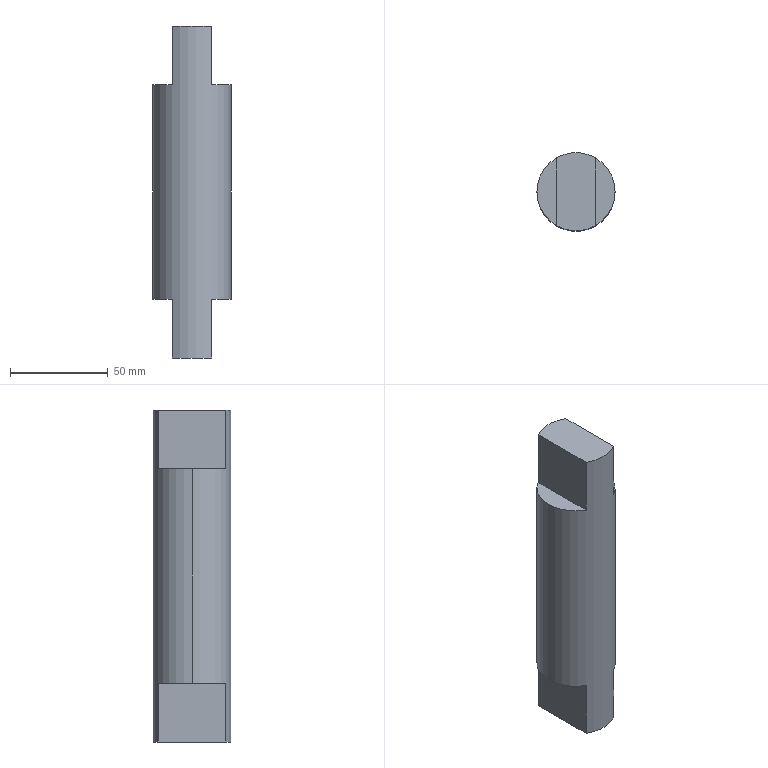Part | SolidWorks | 1 solid | 12 faces | box 40 x 40 x 170 mm | volume 184147 mm3 | plane 10 | cylinder 2 | commonest cylinder face diameters 40 x2
STEP:
#1=CARTESIAN_POINT('',(10.,17.321,0.));
#2=VERTEX_POINT('',#1);
#3=CARTESIAN_POINT('',(20.,0.,0.));
#4=VERTEX_POINT('',#3);
#5=CARTESIAN_POINT('',(0.,0.,0.));
#6=DIRECTION('',(0.,0.,-1.));
#7=DIRECTION('',(-1.,0.,0.));
#8=AXIS2_PLACEMENT_3D('',#5,#6,#7);
#9=CIRCLE('',#8,20.);
#10=EDGE_CURVE('',#2,#4,#9,.T.);
#11=ORIENTED_EDGE('',*,*,#10,.T.);
#12=CARTESIAN_POINT('',(20.,0.,-110.));
#13=VERTEX_POINT('',#12);
#14=CARTESIAN_POINT('',(20.,0.,30.));
#15=DIRECTION('',(0.,0.,-1.));
#16=VECTOR('',#15,1000.);
#17=LINE('',#14,#16);
#18=EDGE_CURVE('',#4,#13,#17,.T.);
#19=ORIENTED_EDGE('',*,*,#18,.T.);
#20=CARTESIAN_POINT('',(10.,17.321,-110.));
#21=VERTEX_POINT('',#20);
#22=CARTESIAN_POINT('',(0.,0.,-110.));
#23=DIRECTION('',(0.,0.,-1.));
#24=DIRECTION('',(-1.,0.,0.));
#25=AXIS2_PLACEMENT_3D('',#22,#23,#24);
#26=CIRCLE('',#25,20.);
#27=EDGE_CURVE('',#21,#13,#26,.T.);
#28=ORIENTED_EDGE('',*,*,#27,.F.);
#29=CARTESIAN_POINT('',(10.,17.321,-140.));
#30=VERTEX_POINT('',#29);
#31=CARTESIAN_POINT('',(10.,17.321,-140.));
#32=DIRECTION('',(0.,0.,1.));
#33=VECTOR('',#32,1000.);
#34=LINE('',#31,#33);
#35=EDGE_CURVE('',#30,#21,#34,.T.);
#36=ORIENTED_EDGE('',*,*,#35,.F.);
#37=CARTESIAN_POINT('',(-10.,17.321,-140.));
#38=VERTEX_POINT('',#37);
#39=CARTESIAN_POINT('',(0.,0.,-140.));
#40=DIRECTION('',(0.,0.,-1.));
#41=DIRECTION('',(-1.,0.,0.));
#42=AXIS2_PLACEMENT_3D('',#39,#40,#41);
#43=CIRCLE('',#42,20.);
#44=EDGE_CURVE('',#38,#30,#43,.T.);
#45=ORIENTED_EDGE('',*,*,#44,.F.);
#46=CARTESIAN_POINT('',(-10.,17.321,-110.));
#47=VERTEX_POINT('',#46);
#48=CARTESIAN_POINT('',(-10.,17.321,-140.));
#49=DIRECTION('',(0.,0.,1.));
#50=VECTOR('',#49,1000.);
#51=LINE('',#48,#50);
#52=EDGE_CURVE('',#38,#47,#51,.T.);
#53=ORIENTED_EDGE('',*,*,#52,.T.);
#54=CARTESIAN_POINT('',(-20.,0.,-110.));
#55=VERTEX_POINT('',#54);
#56=CARTESIAN_POINT('',(0.,0.,-110.));
#57=DIRECTION('',(0.,0.,-1.));
#58=DIRECTION('',(-1.,0.,0.));
#59=AXIS2_PLACEMENT_3D('',#56,#57,#58);
#60=CIRCLE('',#59,20.);
#61=EDGE_CURVE('',#55,#47,#60,.T.);
#62=ORIENTED_EDGE('',*,*,#61,.F.);
#63=CARTESIAN_POINT('',(-20.,0.,0.));
#64=VERTEX_POINT('',#63);
#65=CARTESIAN_POINT('',(-20.,0.,30.));
#66=DIRECTION('',(0.,0.,-1.));
#67=VECTOR('',#66,1000.);
#68=LINE('',#65,#67);
#69=EDGE_CURVE('',#64,#55,#68,.T.);
#70=ORIENTED_EDGE('',*,*,#69,.F.);
#71=CARTESIAN_POINT('',(-10.,17.321,0.));
#72=VERTEX_POINT('',#71);
#73=CARTESIAN_POINT('',(0.,0.,0.));
#74=DIRECTION('',(0.,0.,-1.));
#75=DIRECTION('',(-1.,0.,0.));
#76=AXIS2_PLACEMENT_3D('',#73,#74,#75);
#77=CIRCLE('',#76,20.);
#78=EDGE_CURVE('',#64,#72,#77,.T.);
#79=ORIENTED_EDGE('',*,*,#78,.T.);
#80=CARTESIAN_POINT('',(-10.,17.321,30.));
#81=VERTEX_POINT('',#80);
#82=CARTESIAN_POINT('',(-10.,17.321,30.));
#83=DIRECTION('',(0.,0.,-1.));
#84=VECTOR('',#83,1000.);
#85=LINE('',#82,#84);
#86=EDGE_CURVE('',#81,#72,#85,.T.);
#87=ORIENTED_EDGE('',*,*,#86,.F.);
#88=CARTESIAN_POINT('',(10.,17.321,30.));
#89=VERTEX_POINT('',#88);
#90=CARTESIAN_POINT('',(0.,0.,30.));
#91=DIRECTION('',(0.,0.,1.));
#92=DIRECTION('',(1.,0.,0.));
#93=AXIS2_PLACEMENT_3D('',#90,#91,#92);
#94=CIRCLE('',#93,20.);
#95=EDGE_CURVE('',#89,#81,#94,.T.);
#96=ORIENTED_EDGE('',*,*,#95,.F.);
#97=CARTESIAN_POINT('',(10.,17.321,30.));
#98=DIRECTION('',(0.,0.,-1.));
#99=VECTOR('',#98,1000.);
#100=LINE('',#97,#99);
#101=EDGE_CURVE('',#89,#2,#100,.T.);
#102=ORIENTED_EDGE('',*,*,#101,.T.);
#103=EDGE_LOOP('',(#11,#19,#28,#36,#45,#53,#62,#70,#79,#87,#96,#102));
#104=FACE_OUTER_BOUND('',#103,.T.);
#105=CARTESIAN_POINT('',(0.,0.,30.));
#106=DIRECTION('',(0.,0.,-1.));
#107=DIRECTION('',(-1.,0.,0.));
#108=AXIS2_PLACEMENT_3D('',#105,#106,#107);
#109=CYLINDRICAL_SURFACE('',#108,20.);
#110=ADVANCED_FACE('',(#104),#109,.T.);
#111=CARTESIAN_POINT('',(-10.,-17.321,-110.));
#112=VERTEX_POINT('',#111);
#113=CARTESIAN_POINT('',(0.,0.,-110.));
#114=DIRECTION('',(0.,0.,-1.));
#115=DIRECTION('',(-1.,0.,0.));
#116=AXIS2_PLACEMENT_3D('',#113,#114,#115);
#117=CIRCLE('',#116,20.);
#118=EDGE_CURVE('',#112,#55,#117,.T.);
#119=ORIENTED_EDGE('',*,*,#118,.T.);
#120=ORIENTED_EDGE('',*,*,#61,.T.);
#121=CARTESIAN_POINT('',(-10.,0.,-110.));
#122=DIRECTION('',(0.,-1.,0.));
#123=VECTOR('',#122,1000.);
#124=LINE('',#121,#123);
#125=EDGE_CURVE('',#47,#112,#124,.T.);
#126=ORIENTED_EDGE('',*,*,#125,.T.);
#127=EDGE_LOOP('',(#119,#120,#126));
#128=FACE_OUTER_BOUND('',#127,.T.);
#129=CARTESIAN_POINT('',(0.,0.,-110.));
#130=DIRECTION('',(0.,0.,-1.));
#131=DIRECTION('',(-1.,0.,0.));
#132=AXIS2_PLACEMENT_3D('',#129,#130,#131);
#133=PLANE('',#132);
#134=ADVANCED_FACE('',(#128),#133,.T.);
#135=CARTESIAN_POINT('',(-10.,-17.321,0.));
#136=VERTEX_POINT('',#135);
#137=CARTESIAN_POINT('',(-10.,0.,0.));
#138=DIRECTION('',(0.,-1.,0.));
#139=VECTOR('',#138,1000.);
#140=LINE('',#137,#139);
#141=EDGE_CURVE('',#72,#136,#140,.T.);
#142=ORIENTED_EDGE('',*,*,#141,.T.);
#143=CARTESIAN_POINT('',(-10.,-17.321,30.));
#144=VERTEX_POINT('',#143);
#145=CARTESIAN_POINT('',(-10.,-17.321,30.));
#146=DIRECTION('',(0.,0.,-1.));
#147=VECTOR('',#146,1000.);
#148=LINE('',#145,#147);
#149=EDGE_CURVE('',#144,#136,#148,.T.);
#150=ORIENTED_EDGE('',*,*,#149,.F.);
#151=CARTESIAN_POINT('',(-10.,0.,30.));
#152=DIRECTION('',(0.,-1.,0.));
#153=VECTOR('',#152,1000.);
#154=LINE('',#151,#153);
#155=EDGE_CURVE('',#81,#144,#154,.T.);
#156=ORIENTED_EDGE('',*,*,#155,.F.);
#157=ORIENTED_EDGE('',*,*,#86,.T.);
#158=EDGE_LOOP('',(#142,#150,#156,#157));
#159=FACE_OUTER_BOUND('',#158,.T.);
#160=CARTESIAN_POINT('',(-10.,0.,30.));
#161=DIRECTION('',(1.,0.,0.));
#162=DIRECTION('',(0.,0.,-1.));
#163=AXIS2_PLACEMENT_3D('',#160,#161,#162);
#164=PLANE('',#163);
#165=ADVANCED_FACE('',(#159),#164,.F.);
#166=ORIENTED_EDGE('',*,*,#18,.F.);
#167=CARTESIAN_POINT('',(10.,-17.321,0.));
#168=VERTEX_POINT('',#167);
#169=CARTESIAN_POINT('',(0.,0.,0.));
#170=DIRECTION('',(0.,0.,-1.));
#171=DIRECTION('',(-1.,0.,0.));
#172=AXIS2_PLACEMENT_3D('',#169,#170,#171);
#173=CIRCLE('',#172,20.);
#174=EDGE_CURVE('',#4,#168,#173,.T.);
#175=ORIENTED_EDGE('',*,*,#174,.T.);
#176=CARTESIAN_POINT('',(10.,-17.321,30.));
#177=VERTEX_POINT('',#176);
#178=CARTESIAN_POINT('',(10.,-17.321,30.));
#179=DIRECTION('',(0.,0.,-1.));
#180=VECTOR('',#179,1000.);
#181=LINE('',#178,#180);
#182=EDGE_CURVE('',#177,#168,#181,.T.);
#183=ORIENTED_EDGE('',*,*,#182,.F.);
#184=CARTESIAN_POINT('',(0.,0.,30.));
#185=DIRECTION('',(0.,0.,1.));
#186=DIRECTION('',(1.,0.,0.));
#187=AXIS2_PLACEMENT_3D('',#184,#185,#186);
#188=CIRCLE('',#187,20.);
#189=EDGE_CURVE('',#144,#177,#188,.T.);
#190=ORIENTED_EDGE('',*,*,#189,.F.);
#191=ORIENTED_EDGE('',*,*,#149,.T.);
#192=CARTESIAN_POINT('',(0.,0.,0.));
#193=DIRECTION('',(0.,0.,-1.));
#194=DIRECTION('',(-1.,0.,0.));
#195=AXIS2_PLACEMENT_3D('',#192,#193,#194);
#196=CIRCLE('',#195,20.);
#197=EDGE_CURVE('',#136,#64,#196,.T.);
#198=ORIENTED_EDGE('',*,*,#197,.T.);
#199=ORIENTED_EDGE('',*,*,#69,.T.);
#200=ORIENTED_EDGE('',*,*,#118,.F.);
#201=CARTESIAN_POINT('',(-10.,-17.321,-140.));
#202=VERTEX_POINT('',#201);
#203=CARTESIAN_POINT('',(-10.,-17.321,-140.));
#204=DIRECTION('',(0.,0.,1.));
#205=VECTOR('',#204,1000.);
#206=LINE('',#203,#205);
#207=EDGE_CURVE('',#202,#112,#206,.T.);
#208=ORIENTED_EDGE('',*,*,#207,.F.);
#209=CARTESIAN_POINT('',(10.,-17.321,-140.));
#210=VERTEX_POINT('',#209);
#211=CARTESIAN_POINT('',(0.,0.,-140.));
#212=DIRECTION('',(0.,0.,-1.));
#213=DIRECTION('',(-1.,0.,0.));
#214=AXIS2_PLACEMENT_3D('',#211,#212,#213);
#215=CIRCLE('',#214,20.);
#216=EDGE_CURVE('',#210,#202,#215,.T.);
#217=ORIENTED_EDGE('',*,*,#216,.F.);
#218=CARTESIAN_POINT('',(10.,-17.321,-110.));
#219=VERTEX_POINT('',#218);
#220=CARTESIAN_POINT('',(10.,-17.321,-140.));
#221=DIRECTION('',(0.,0.,1.));
#222=VECTOR('',#221,1000.);
#223=LINE('',#220,#222);
#224=EDGE_CURVE('',#210,#219,#223,.T.);
#225=ORIENTED_EDGE('',*,*,#224,.T.);
#226=CARTESIAN_POINT('',(0.,0.,-110.));
#227=DIRECTION('',(0.,0.,-1.));
#228=DIRECTION('',(-1.,0.,0.));
#229=AXIS2_PLACEMENT_3D('',#226,#227,#228);
#230=CIRCLE('',#229,20.);
#231=EDGE_CURVE('',#13,#219,#230,.T.);
#232=ORIENTED_EDGE('',*,*,#231,.F.);
#233=EDGE_LOOP('',(#166,#175,#183,#190,#191,#198,#199,#200,#208,#217,#225,#232));
#234=FACE_OUTER_BOUND('',#233,.T.);
#235=CARTESIAN_POINT('',(0.,0.,30.));
#236=DIRECTION('',(0.,0.,-1.));
#237=DIRECTION('',(-1.,0.,0.));
#238=AXIS2_PLACEMENT_3D('',#235,#236,#237);
#239=CYLINDRICAL_SURFACE('',#238,20.);
#240=ADVANCED_FACE('',(#234),#239,.T.);
#241=CARTESIAN_POINT('',(10.,0.,0.));
#242=DIRECTION('',(0.,-1.,0.));
#243=VECTOR('',#242,1000.);
#244=LINE('',#241,#243);
#245=EDGE_CURVE('',#2,#168,#244,.T.);
#246=ORIENTED_EDGE('',*,*,#245,.F.);
#247=ORIENTED_EDGE('',*,*,#101,.F.);
#248=CARTESIAN_POINT('',(10.,0.,30.));
#249=DIRECTION('',(0.,-1.,0.));
#250=VECTOR('',#249,1000.);
#251=LINE('',#248,#250);
#252=EDGE_CURVE('',#89,#177,#251,.T.);
#253=ORIENTED_EDGE('',*,*,#252,.T.);
#254=ORIENTED_EDGE('',*,*,#182,.T.);
#255=EDGE_LOOP('',(#246,#247,#253,#254));
#256=FACE_OUTER_BOUND('',#255,.T.);
#257=CARTESIAN_POINT('',(10.,0.,30.));
#258=DIRECTION('',(1.,0.,0.));
#259=DIRECTION('',(0.,0.,-1.));
#260=AXIS2_PLACEMENT_3D('',#257,#258,#259);
#261=PLANE('',#260);
#262=ADVANCED_FACE('',(#256),#261,.T.);
#263=ORIENTED_EDGE('',*,*,#95,.T.);
#264=ORIENTED_EDGE('',*,*,#155,.T.);
#265=ORIENTED_EDGE('',*,*,#189,.T.);
#266=ORIENTED_EDGE('',*,*,#252,.F.);
#267=EDGE_LOOP('',(#263,#264,#265,#266));
#268=FACE_OUTER_BOUND('',#267,.T.);
#269=CARTESIAN_POINT('',(0.,0.,30.));
#270=DIRECTION('',(0.,0.,1.));
#271=DIRECTION('',(1.,0.,0.));
#272=AXIS2_PLACEMENT_3D('',#269,#270,#271);
#273=PLANE('',#272);
#274=ADVANCED_FACE('',(#268),#273,.T.);
#275=ORIENTED_EDGE('',*,*,#10,.F.);
#276=ORIENTED_EDGE('',*,*,#245,.T.);
#277=ORIENTED_EDGE('',*,*,#174,.F.);
#278=EDGE_LOOP('',(#275,#276,#277));
#279=FACE_OUTER_BOUND('',#278,.T.);
#280=CARTESIAN_POINT('',(0.,0.,0.));
#281=DIRECTION('',(0.,0.,-1.));
#282=DIRECTION('',(-1.,0.,0.));
#283=AXIS2_PLACEMENT_3D('',#280,#281,#282);
#284=PLANE('',#283);
#285=ADVANCED_FACE('',(#279),#284,.F.);
#286=CARTESIAN_POINT('',(10.,0.,-110.));
#287=DIRECTION('',(0.,-1.,0.));
#288=VECTOR('',#287,1000.);
#289=LINE('',#286,#288);
#290=EDGE_CURVE('',#21,#219,#289,.T.);
#291=ORIENTED_EDGE('',*,*,#290,.F.);
#292=ORIENTED_EDGE('',*,*,#27,.T.);
#293=ORIENTED_EDGE('',*,*,#231,.T.);
#294=EDGE_LOOP('',(#291,#292,#293));
#295=FACE_OUTER_BOUND('',#294,.T.);
#296=CARTESIAN_POINT('',(0.,0.,-110.));
#297=DIRECTION('',(0.,0.,-1.));
#298=DIRECTION('',(-1.,0.,0.));
#299=AXIS2_PLACEMENT_3D('',#296,#297,#298);
#300=PLANE('',#299);
#301=ADVANCED_FACE('',(#295),#300,.T.);
#302=ORIENTED_EDGE('',*,*,#141,.F.);
#303=ORIENTED_EDGE('',*,*,#78,.F.);
#304=ORIENTED_EDGE('',*,*,#197,.F.);
#305=EDGE_LOOP('',(#302,#303,#304));
#306=FACE_OUTER_BOUND('',#305,.T.);
#307=CARTESIAN_POINT('',(0.,0.,0.));
#308=DIRECTION('',(0.,0.,-1.));
#309=DIRECTION('',(-1.,0.,0.));
#310=AXIS2_PLACEMENT_3D('',#307,#308,#309);
#311=PLANE('',#310);
#312=ADVANCED_FACE('',(#306),#311,.F.);
#313=ORIENTED_EDGE('',*,*,#290,.T.);
#314=ORIENTED_EDGE('',*,*,#224,.F.);
#315=CARTESIAN_POINT('',(10.,0.,-140.));
#316=DIRECTION('',(0.,-1.,0.));
#317=VECTOR('',#316,1000.);
#318=LINE('',#315,#317);
#319=EDGE_CURVE('',#30,#210,#318,.T.);
#320=ORIENTED_EDGE('',*,*,#319,.F.);
#321=ORIENTED_EDGE('',*,*,#35,.T.);
#322=EDGE_LOOP('',(#313,#314,#320,#321));
#323=FACE_OUTER_BOUND('',#322,.T.);
#324=CARTESIAN_POINT('',(10.,0.,-140.));
#325=DIRECTION('',(-1.,0.,0.));
#326=DIRECTION('',(0.,0.,1.));
#327=AXIS2_PLACEMENT_3D('',#324,#325,#326);
#328=PLANE('',#327);
#329=ADVANCED_FACE('',(#323),#328,.F.);
#330=ORIENTED_EDGE('',*,*,#125,.F.);
#331=ORIENTED_EDGE('',*,*,#52,.F.);
#332=CARTESIAN_POINT('',(-10.,0.,-140.));
#333=DIRECTION('',(0.,-1.,0.));
#334=VECTOR('',#333,1000.);
#335=LINE('',#332,#334);
#336=EDGE_CURVE('',#38,#202,#335,.T.);
#337=ORIENTED_EDGE('',*,*,#336,.T.);
#338=ORIENTED_EDGE('',*,*,#207,.T.);
#339=EDGE_LOOP('',(#330,#331,#337,#338));
#340=FACE_OUTER_BOUND('',#339,.T.);
#341=CARTESIAN_POINT('',(-10.,0.,-140.));
#342=DIRECTION('',(-1.,0.,0.));
#343=DIRECTION('',(0.,0.,1.));
#344=AXIS2_PLACEMENT_3D('',#341,#342,#343);
#345=PLANE('',#344);
#346=ADVANCED_FACE('',(#340),#345,.T.);
#347=ORIENTED_EDGE('',*,*,#44,.T.);
#348=ORIENTED_EDGE('',*,*,#319,.T.);
#349=ORIENTED_EDGE('',*,*,#216,.T.);
#350=ORIENTED_EDGE('',*,*,#336,.F.);
#351=EDGE_LOOP('',(#347,#348,#349,#350));
#352=FACE_OUTER_BOUND('',#351,.T.);
#353=CARTESIAN_POINT('',(0.,0.,-140.));
#354=DIRECTION('',(0.,0.,-1.));
#355=DIRECTION('',(-1.,0.,0.));
#356=AXIS2_PLACEMENT_3D('',#353,#354,#355);
#357=PLANE('',#356);
#358=ADVANCED_FACE('',(#352),#357,.T.);
#359=CLOSED_SHELL('',(#110,#134,#165,#240,#262,#274,#285,#301,#312,#329,#346,#358));
#360=MANIFOLD_SOLID_BREP('',#359);
#361=CARTESIAN_POINT('',(0.,0.,0.));
#362=DIRECTION('',(0.,0.,1.));
#363=DIRECTION('',(1.,0.,0.));
#364=AXIS2_PLACEMENT_3D('',#361,#362,#363);
#365=(LENGTH_UNIT()NAMED_UNIT(*)SI_UNIT(.MILLI.,.METRE.));
#366=UNCERTAINTY_MEASURE_WITH_UNIT(LENGTH_MEASURE(0.00001),#365,'','');
#367=(NAMED_UNIT(*)PLANE_ANGLE_UNIT()SI_UNIT($,.RADIAN.));
#368=(NAMED_UNIT(*)SI_UNIT($,.STERADIAN.)SOLID_ANGLE_UNIT());
#369=(GEOMETRIC_REPRESENTATION_CONTEXT(3)GLOBAL_UNCERTAINTY_ASSIGNED_CONTEXT((#366))GLOBAL_UNIT_ASSIGNED_CONTEXT((#365,#367,#368))REPRESENTATION_CONTEXT('',''));
#370=ADVANCED_BREP_SHAPE_REPRESENTATION('',(#360,#364),#369);